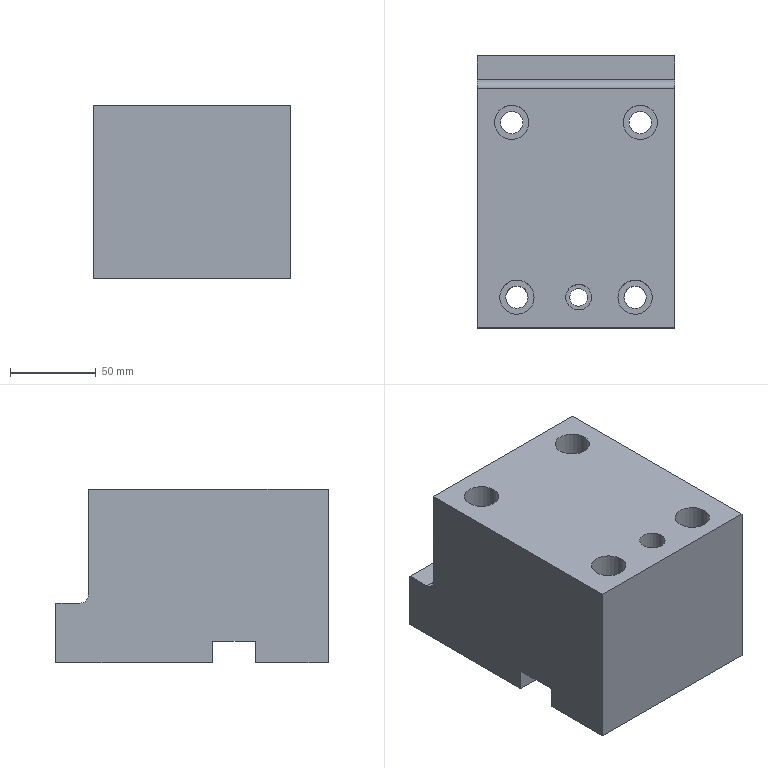Part | STEP file | 1_id1610_x_t | 1 solid | 38 faces | box 115 x 159 x 101.122 mm | volume 1560296 mm3 | plane 17 | cylinder 15 | cone 6 | commonest cylinder face diameters 13 x4 20 x4 6.75 x2 7.938 x2 10 x1 10.25 x1